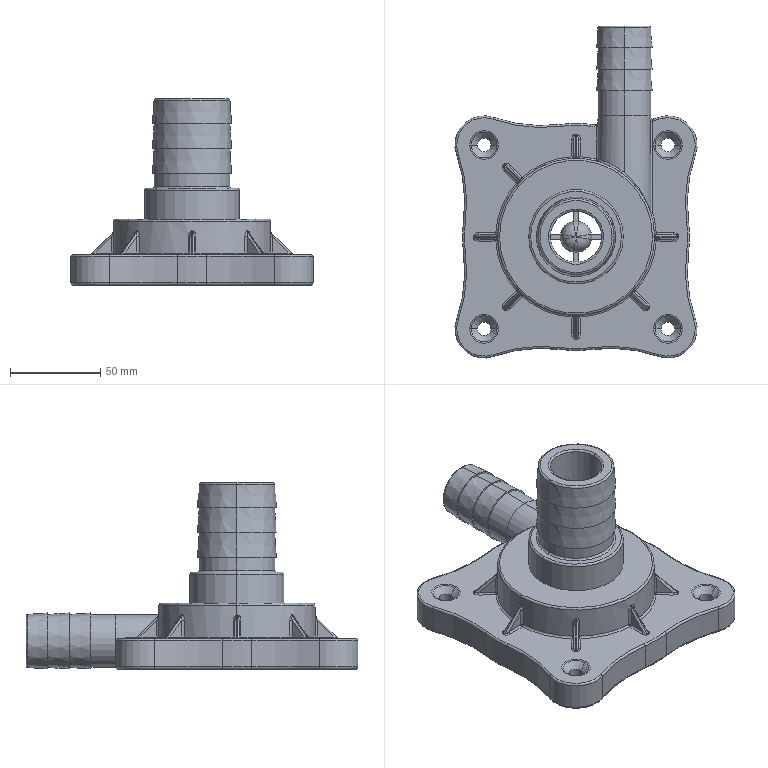Part | SolidWorks | features BaseBody 3 | 3 solids | 367 faces | box 134.4 x 184.2 x 103.29 mm | volume 334800 mm3 | cylinder 103 | torus 90 | spline 59 | plane 56 | sphere 32 | cone 27 | commonest cylinder face diameters 2.1 x30 162 x9 2.4 x8 7.5 x8 17.4 x8 33 x8